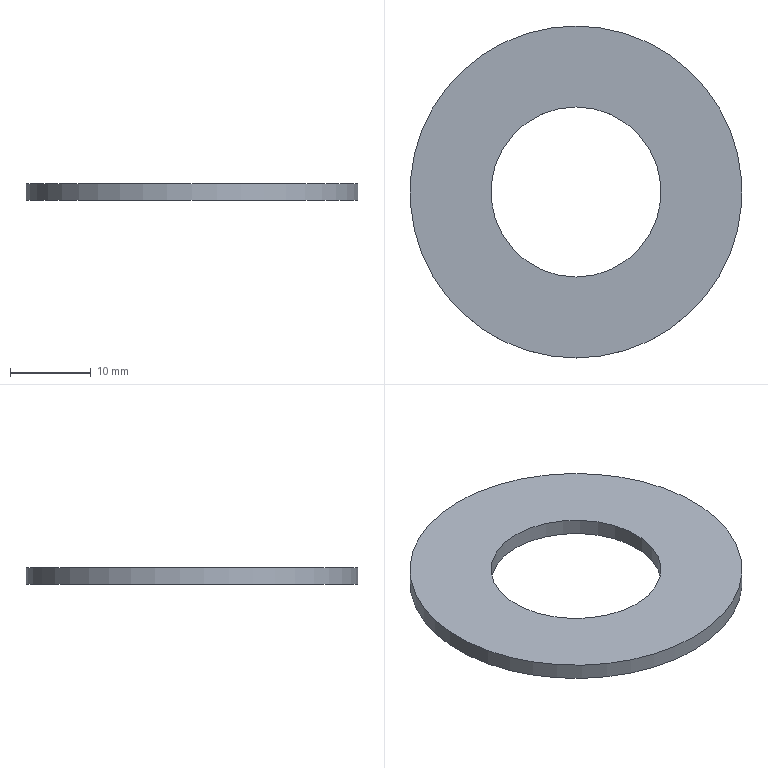Part | NX | features solid 2 | 1 solid | 4 faces | box 41 x 41 x 2 mm | volume 1948 mm3 | cylinder 2 | plane 2 | commonest cylinder face diameters 21 x1 41 x1
STEP:
#1=CARTESIAN_POINT('',(-652.5,-119.5,-53.));
#2=VERTEX_POINT('',#1);
#3=CARTESIAN_POINT('',(-652.5,-140.,-53.));
#4=DIRECTION('',(0.,0.,1.));
#5=DIRECTION('',(0.,1.,0.));
#6=AXIS2_PLACEMENT_3D('',#3,#4,#5);
#7=CIRCLE('',#6,20.5);
#8=EDGE_CURVE('',#2,#2,#7,.T.);
#9=ORIENTED_EDGE('',*,*,#8,.F.);
#10=EDGE_LOOP('',(#9));
#11=FACE_BOUND('',#10,.T.);
#12=CARTESIAN_POINT('',(-652.5,-119.5,-55.));
#13=VERTEX_POINT('',#12);
#14=CARTESIAN_POINT('',(-652.5,-140.,-55.));
#15=DIRECTION('',(0.,0.,1.));
#16=DIRECTION('',(0.,1.,0.));
#17=AXIS2_PLACEMENT_3D('',#14,#15,#16);
#18=CIRCLE('',#17,20.5);
#19=EDGE_CURVE('',#13,#13,#18,.T.);
#20=ORIENTED_EDGE('',*,*,#19,.T.);
#21=EDGE_LOOP('',(#20));
#22=FACE_BOUND('',#21,.T.);
#23=CARTESIAN_POINT('',(-652.5,-140.,-55.));
#24=DIRECTION('',(0.,0.,1.));
#25=DIRECTION('',(0.,1.,0.));
#26=AXIS2_PLACEMENT_3D('',#23,#24,#25);
#27=CYLINDRICAL_SURFACE('',#26,20.5);
#28=ADVANCED_FACE('',(#11,#22),#27,.T.);
#29=ORIENTED_EDGE('',*,*,#19,.F.);
#30=EDGE_LOOP('',(#29));
#31=FACE_BOUND('',#30,.T.);
#32=CARTESIAN_POINT('',(-652.5,-129.5,-55.));
#33=VERTEX_POINT('',#32);
#34=CARTESIAN_POINT('',(-652.5,-140.,-55.));
#35=DIRECTION('',(0.,0.,1.));
#36=DIRECTION('',(0.,1.,0.));
#37=AXIS2_PLACEMENT_3D('',#34,#35,#36);
#38=CIRCLE('',#37,10.5);
#39=EDGE_CURVE('',#33,#33,#38,.T.);
#40=ORIENTED_EDGE('',*,*,#39,.T.);
#41=EDGE_LOOP('',(#40));
#42=FACE_BOUND('',#41,.T.);
#43=CARTESIAN_POINT('',(-652.5,-140.,-55.));
#44=DIRECTION('',(0.,0.,-1.));
#45=DIRECTION('',(0.,-1.,0.));
#46=AXIS2_PLACEMENT_3D('',#43,#44,#45);
#47=PLANE('',#46);
#48=ADVANCED_FACE('',(#31,#42),#47,.T.);
#49=ORIENTED_EDGE('',*,*,#8,.T.);
#50=EDGE_LOOP('',(#49));
#51=FACE_BOUND('',#50,.T.);
#52=CARTESIAN_POINT('',(-652.5,-129.5,-53.));
#53=VERTEX_POINT('',#52);
#54=CARTESIAN_POINT('',(-652.5,-140.,-53.));
#55=DIRECTION('',(0.,0.,1.));
#56=DIRECTION('',(0.,1.,0.));
#57=AXIS2_PLACEMENT_3D('',#54,#55,#56);
#58=CIRCLE('',#57,10.5);
#59=EDGE_CURVE('',#53,#53,#58,.T.);
#60=ORIENTED_EDGE('',*,*,#59,.F.);
#61=EDGE_LOOP('',(#60));
#62=FACE_BOUND('',#61,.T.);
#63=CARTESIAN_POINT('',(-652.5,-140.,-53.));
#64=DIRECTION('',(0.,0.,-1.));
#65=DIRECTION('',(0.,-1.,0.));
#66=AXIS2_PLACEMENT_3D('',#63,#64,#65);
#67=PLANE('',#66);
#68=ADVANCED_FACE('',(#51,#62),#67,.F.);
#69=ORIENTED_EDGE('',*,*,#59,.T.);
#70=EDGE_LOOP('',(#69));
#71=FACE_BOUND('',#70,.T.);
#72=ORIENTED_EDGE('',*,*,#39,.F.);
#73=EDGE_LOOP('',(#72));
#74=FACE_BOUND('',#73,.T.);
#75=CARTESIAN_POINT('',(-652.5,-140.,-55.));
#76=DIRECTION('',(0.,0.,1.));
#77=DIRECTION('',(0.,1.,0.));
#78=AXIS2_PLACEMENT_3D('',#75,#76,#77);
#79=CYLINDRICAL_SURFACE('',#78,10.5);
#80=ADVANCED_FACE('',(#71,#74),#79,.F.);
#81=CLOSED_SHELL('',(#28,#48,#68,#80));
#82=MANIFOLD_SOLID_BREP('',#81);
#83=(LENGTH_UNIT()NAMED_UNIT(*)SI_UNIT(.MILLI.,.METRE.));
#84=UNCERTAINTY_MEASURE_WITH_UNIT(LENGTH_MEASURE(0.00001),#83,'','');
#85=(NAMED_UNIT(*)PLANE_ANGLE_UNIT()SI_UNIT($,.RADIAN.));
#86=(NAMED_UNIT(*)SI_UNIT($,.STERADIAN.)SOLID_ANGLE_UNIT());
#87=(GEOMETRIC_REPRESENTATION_CONTEXT(3)GLOBAL_UNCERTAINTY_ASSIGNED_CONTEXT((#84))GLOBAL_UNIT_ASSIGNED_CONTEXT((#83,#85,#86))REPRESENTATION_CONTEXT('',''));
#88=ADVANCED_BREP_SHAPE_REPRESENTATION('',(#82),#87);